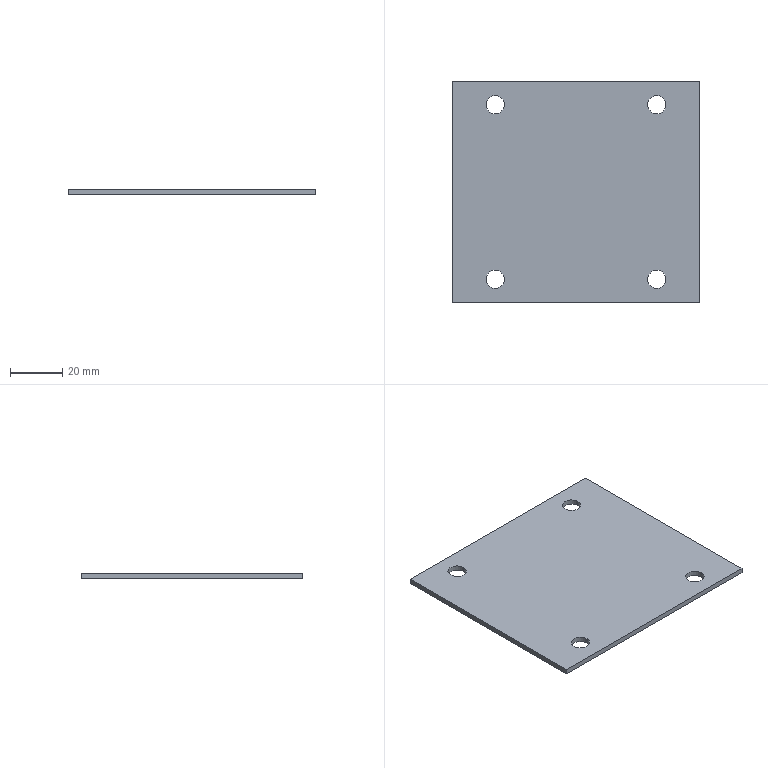Part | STEP file | GLSJ-10-47 | 1 solid | 14 faces | box 95 x 85 x 2 mm | volume 15842 mm3 | cylinder 8 | plane 6 | commonest cylinder face diameters 7 x8
STEP:
#1=CARTESIAN_POINT('',(0.,0.,0.));
#2=DIRECTION('',(0.,0.,1.));
#3=DIRECTION('',(1.,0.,0.));
#4=AXIS2_PLACEMENT_3D('',#1,#2,#3);
#5=CARTESIAN_POINT('',(-27.5,-33.5,0.));
#6=VERTEX_POINT('',#5);
#7=CARTESIAN_POINT('',(-27.5,-33.5,2.));
#8=VERTEX_POINT('',#7);
#9=CARTESIAN_POINT('',(-27.5,-33.5,0.));
#10=DIRECTION('',(0.,0.,1.));
#11=VECTOR('',#10,1.);
#12=LINE('',#9,#11);
#13=CARTESIAN_POINT('',(-31.,-33.5,0.));
#14=DIRECTION('',(0.,0.,1.));
#15=DIRECTION('',(1.,0.,0.));
#16=AXIS2_PLACEMENT_3D('',#13,#14,#15);
#17=CYLINDRICAL_SURFACE('',#16,3.5);
#18=CARTESIAN_POINT('',(6.283,0.));
#19=DIRECTION('',(0.,1.));
#20=VECTOR('',#19,1.);
#21=LINE('',#18,#20);
#22=(GEOMETRIC_REPRESENTATION_CONTEXT(2)PARAMETRIC_REPRESENTATION_CONTEXT()REPRESENTATION_CONTEXT('',''));
#23=DEFINITIONAL_REPRESENTATION('',(#21),#22);
#24=PCURVE('',#17,#23);
#25=CARTESIAN_POINT('',(-31.,-33.5,0.));
#26=DIRECTION('',(0.,0.,1.));
#27=DIRECTION('',(1.,0.,0.));
#28=AXIS2_PLACEMENT_3D('',#25,#26,#27);
#29=CYLINDRICAL_SURFACE('',#28,3.5);
#30=CARTESIAN_POINT('',(0.,0.));
#31=DIRECTION('',(0.,1.));
#32=VECTOR('',#31,1.);
#33=LINE('',#30,#32);
#34=(GEOMETRIC_REPRESENTATION_CONTEXT(2)PARAMETRIC_REPRESENTATION_CONTEXT()REPRESENTATION_CONTEXT('',''));
#35=DEFINITIONAL_REPRESENTATION('',(#33),#34);
#36=PCURVE('',#29,#35);
#37=SURFACE_CURVE('',#12,(#24,#36),.PCURVE_S1.);
#38=EDGE_CURVE('',#6,#8,#37,.T.);
#39=ORIENTED_EDGE('',*,*,#38,.T.);
#40=CARTESIAN_POINT('',(-34.5,-33.5,2.));
#41=VERTEX_POINT('',#40);
#42=CARTESIAN_POINT('',(-31.,-33.5,2.));
#43=DIRECTION('',(0.,0.,1.));
#44=DIRECTION('',(-1.,0.,0.));
#45=AXIS2_PLACEMENT_3D('',#42,#43,#44);
#46=CIRCLE('',#45,3.5);
#47=CARTESIAN_POINT('',(3.142,2.));
#48=DIRECTION('',(1.,0.));
#49=VECTOR('',#48,1.);
#50=LINE('',#47,#49);
#51=(GEOMETRIC_REPRESENTATION_CONTEXT(2)PARAMETRIC_REPRESENTATION_CONTEXT()REPRESENTATION_CONTEXT('',''));
#52=DEFINITIONAL_REPRESENTATION('',(#50),#51);
#53=PCURVE('',#17,#52);
#54=CARTESIAN_POINT('',(0.,0.,2.));
#55=DIRECTION('',(0.,0.,-1.));
#56=DIRECTION('',(-1.,0.,0.));
#57=AXIS2_PLACEMENT_3D('',#54,#55,#56);
#58=PLANE('',#57);
#59=CARTESIAN_POINT('',(34.5,-33.5));
#60=CARTESIAN_POINT('',(34.5,-39.562));
#61=CARTESIAN_POINT('',(29.25,-36.531));
#62=CARTESIAN_POINT('',(24.,-33.5));
#63=CARTESIAN_POINT('',(29.25,-30.469));
#64=CARTESIAN_POINT('',(34.5,-27.438));
#65=CARTESIAN_POINT('',(34.5,-33.5));
#66=(BOUNDED_CURVE()B_SPLINE_CURVE(2,(#59,#60,#61,#62,#63,#64,#65),.UNSPECIFIED.,.T.,.F.)B_SPLINE_CURVE_WITH_KNOTS((1,2,2,2,2,1),(-2.094,0.,2.094,4.189,6.283,8.378),.UNSPECIFIED.)CURVE()GEOMETRIC_REPRESENTATION_ITEM()RATIONAL_B_SPLINE_CURVE((1.,0.5,1.,0.5,1.,0.5,1.))REPRESENTATION_ITEM(''));
#67=(GEOMETRIC_REPRESENTATION_CONTEXT(2)PARAMETRIC_REPRESENTATION_CONTEXT()REPRESENTATION_CONTEXT('',''));
#68=DEFINITIONAL_REPRESENTATION('',(#66),#67);
#69=PCURVE('',#58,#68);
#70=SURFACE_CURVE('',#46,(#53,#69),.PCURVE_S1.);
#71=EDGE_CURVE('',#41,#8,#70,.T.);
#72=ORIENTED_EDGE('',*,*,#71,.F.);
#73=CARTESIAN_POINT('',(-34.5,-33.5,0.));
#74=VERTEX_POINT('',#73);
#75=CARTESIAN_POINT('',(-34.5,-33.5,0.));
#76=DIRECTION('',(0.,0.,1.));
#77=VECTOR('',#76,1.);
#78=LINE('',#75,#77);
#79=CARTESIAN_POINT('',(3.142,0.));
#80=DIRECTION('',(0.,1.));
#81=VECTOR('',#80,1.);
#82=LINE('',#79,#81);
#83=(GEOMETRIC_REPRESENTATION_CONTEXT(2)PARAMETRIC_REPRESENTATION_CONTEXT()REPRESENTATION_CONTEXT('',''));
#84=DEFINITIONAL_REPRESENTATION('',(#82),#83);
#85=PCURVE('',#17,#84);
#86=CARTESIAN_POINT('',(3.142,0.));
#87=DIRECTION('',(0.,1.));
#88=VECTOR('',#87,1.);
#89=LINE('',#86,#88);
#90=(GEOMETRIC_REPRESENTATION_CONTEXT(2)PARAMETRIC_REPRESENTATION_CONTEXT()REPRESENTATION_CONTEXT('',''));
#91=DEFINITIONAL_REPRESENTATION('',(#89),#90);
#92=PCURVE('',#29,#91);
#93=SURFACE_CURVE('',#78,(#85,#92),.PCURVE_S1.);
#94=EDGE_CURVE('',#74,#41,#93,.T.);
#95=ORIENTED_EDGE('',*,*,#94,.F.);
#96=CARTESIAN_POINT('',(-31.,-33.5,0.));
#97=DIRECTION('',(0.,0.,1.));
#98=DIRECTION('',(-1.,0.,0.));
#99=AXIS2_PLACEMENT_3D('',#96,#97,#98);
#100=CIRCLE('',#99,3.5);
#101=CARTESIAN_POINT('',(3.142,0.));
#102=DIRECTION('',(1.,0.));
#103=VECTOR('',#102,1.);
#104=LINE('',#101,#103);
#105=(GEOMETRIC_REPRESENTATION_CONTEXT(2)PARAMETRIC_REPRESENTATION_CONTEXT()REPRESENTATION_CONTEXT('',''));
#106=DEFINITIONAL_REPRESENTATION('',(#104),#105);
#107=PCURVE('',#17,#106);
#108=CARTESIAN_POINT('',(0.,0.,0.));
#109=DIRECTION('',(0.,0.,-1.));
#110=DIRECTION('',(-1.,0.,0.));
#111=AXIS2_PLACEMENT_3D('',#108,#109,#110);
#112=PLANE('',#111);
#113=CARTESIAN_POINT('',(34.5,-33.5));
#114=CARTESIAN_POINT('',(34.5,-39.562));
#115=CARTESIAN_POINT('',(29.25,-36.531));
#116=CARTESIAN_POINT('',(24.,-33.5));
#117=CARTESIAN_POINT('',(29.25,-30.469));
#118=CARTESIAN_POINT('',(34.5,-27.438));
#119=CARTESIAN_POINT('',(34.5,-33.5));
#120=(BOUNDED_CURVE()B_SPLINE_CURVE(2,(#113,#114,#115,#116,#117,#118,#119),.UNSPECIFIED.,.T.,.F.)B_SPLINE_CURVE_WITH_KNOTS((1,2,2,2,2,1),(-2.094,0.,2.094,4.189,6.283,8.378),.UNSPECIFIED.)CURVE()GEOMETRIC_REPRESENTATION_ITEM()RATIONAL_B_SPLINE_CURVE((1.,0.5,1.,0.5,1.,0.5,1.))REPRESENTATION_ITEM(''));
#121=(GEOMETRIC_REPRESENTATION_CONTEXT(2)PARAMETRIC_REPRESENTATION_CONTEXT()REPRESENTATION_CONTEXT('',''));
#122=DEFINITIONAL_REPRESENTATION('',(#120),#121);
#123=PCURVE('',#112,#122);
#124=SURFACE_CURVE('',#100,(#107,#123),.PCURVE_S1.);
#125=EDGE_CURVE('',#74,#6,#124,.T.);
#126=ORIENTED_EDGE('',*,*,#125,.T.);
#127=EDGE_LOOP('',(#39,#72,#95,#126));
#128=FACE_BOUND('',#127,.F.);
#129=ADVANCED_FACE('',(#128),#17,.F.);
#130=CARTESIAN_POINT('',(34.5,-33.5,0.));
#131=VERTEX_POINT('',#130);
#132=CARTESIAN_POINT('',(34.5,-33.5,2.));
#133=VERTEX_POINT('',#132);
#134=CARTESIAN_POINT('',(34.5,-33.5,0.));
#135=DIRECTION('',(0.,0.,1.));
#136=VECTOR('',#135,1.);
#137=LINE('',#134,#136);
#138=CARTESIAN_POINT('',(31.,-33.5,0.));
#139=DIRECTION('',(0.,0.,1.));
#140=DIRECTION('',(1.,0.,0.));
#141=AXIS2_PLACEMENT_3D('',#138,#139,#140);
#142=CYLINDRICAL_SURFACE('',#141,3.5);
#143=CARTESIAN_POINT('',(6.283,0.));
#144=DIRECTION('',(0.,1.));
#145=VECTOR('',#144,1.);
#146=LINE('',#143,#145);
#147=(GEOMETRIC_REPRESENTATION_CONTEXT(2)PARAMETRIC_REPRESENTATION_CONTEXT()REPRESENTATION_CONTEXT('',''));
#148=DEFINITIONAL_REPRESENTATION('',(#146),#147);
#149=PCURVE('',#142,#148);
#150=CARTESIAN_POINT('',(31.,-33.5,0.));
#151=DIRECTION('',(0.,0.,1.));
#152=DIRECTION('',(1.,0.,0.));
#153=AXIS2_PLACEMENT_3D('',#150,#151,#152);
#154=CYLINDRICAL_SURFACE('',#153,3.5);
#155=CARTESIAN_POINT('',(0.,0.));
#156=DIRECTION('',(0.,1.));
#157=VECTOR('',#156,1.);
#158=LINE('',#155,#157);
#159=(GEOMETRIC_REPRESENTATION_CONTEXT(2)PARAMETRIC_REPRESENTATION_CONTEXT()REPRESENTATION_CONTEXT('',''));
#160=DEFINITIONAL_REPRESENTATION('',(#158),#159);
#161=PCURVE('',#154,#160);
#162=SURFACE_CURVE('',#137,(#149,#161),.PCURVE_S1.);
#163=EDGE_CURVE('',#131,#133,#162,.T.);
#164=ORIENTED_EDGE('',*,*,#163,.T.);
#165=CARTESIAN_POINT('',(27.5,-33.5,2.));
#166=VERTEX_POINT('',#165);
#167=CARTESIAN_POINT('',(31.,-33.5,2.));
#168=DIRECTION('',(0.,0.,1.));
#169=DIRECTION('',(1.,0.,0.));
#170=AXIS2_PLACEMENT_3D('',#167,#168,#169);
#171=CIRCLE('',#170,3.5);
#172=CARTESIAN_POINT('',(0.,2.));
#173=DIRECTION('',(1.,0.));
#174=VECTOR('',#173,1.);
#175=LINE('',#172,#174);
#176=(GEOMETRIC_REPRESENTATION_CONTEXT(2)PARAMETRIC_REPRESENTATION_CONTEXT()REPRESENTATION_CONTEXT('',''));
#177=DEFINITIONAL_REPRESENTATION('',(#175),#176);
#178=PCURVE('',#142,#177);
#179=CARTESIAN_POINT('',(-34.5,-33.5));
#180=CARTESIAN_POINT('',(-34.5,-27.438));
#181=CARTESIAN_POINT('',(-29.25,-30.469));
#182=CARTESIAN_POINT('',(-24.,-33.5));
#183=CARTESIAN_POINT('',(-29.25,-36.531));
#184=CARTESIAN_POINT('',(-34.5,-39.562));
#185=CARTESIAN_POINT('',(-34.5,-33.5));
#186=(BOUNDED_CURVE()B_SPLINE_CURVE(2,(#179,#180,#181,#182,#183,#184,#185),.UNSPECIFIED.,.T.,.F.)B_SPLINE_CURVE_WITH_KNOTS((1,2,2,2,2,1),(-2.094,0.,2.094,4.189,6.283,8.378),.UNSPECIFIED.)CURVE()GEOMETRIC_REPRESENTATION_ITEM()RATIONAL_B_SPLINE_CURVE((1.,0.5,1.,0.5,1.,0.5,1.))REPRESENTATION_ITEM(''));
#187=(GEOMETRIC_REPRESENTATION_CONTEXT(2)PARAMETRIC_REPRESENTATION_CONTEXT()REPRESENTATION_CONTEXT('',''));
#188=DEFINITIONAL_REPRESENTATION('',(#186),#187);
#189=PCURVE('',#58,#188);
#190=SURFACE_CURVE('',#171,(#178,#189),.PCURVE_S1.);
#191=EDGE_CURVE('',#166,#133,#190,.T.);
#192=ORIENTED_EDGE('',*,*,#191,.F.);
#193=CARTESIAN_POINT('',(27.5,-33.5,0.));
#194=VERTEX_POINT('',#193);
#195=CARTESIAN_POINT('',(27.5,-33.5,0.));
#196=DIRECTION('',(0.,0.,1.));
#197=VECTOR('',#196,1.);
#198=LINE('',#195,#197);
#199=CARTESIAN_POINT('',(3.142,0.));
#200=DIRECTION('',(0.,1.));
#201=VECTOR('',#200,1.);
#202=LINE('',#199,#201);
#203=(GEOMETRIC_REPRESENTATION_CONTEXT(2)PARAMETRIC_REPRESENTATION_CONTEXT()REPRESENTATION_CONTEXT('',''));
#204=DEFINITIONAL_REPRESENTATION('',(#202),#203);
#205=PCURVE('',#142,#204);
#206=CARTESIAN_POINT('',(3.142,0.));
#207=DIRECTION('',(0.,1.));
#208=VECTOR('',#207,1.);
#209=LINE('',#206,#208);
#210=(GEOMETRIC_REPRESENTATION_CONTEXT(2)PARAMETRIC_REPRESENTATION_CONTEXT()REPRESENTATION_CONTEXT('',''));
#211=DEFINITIONAL_REPRESENTATION('',(#209),#210);
#212=PCURVE('',#154,#211);
#213=SURFACE_CURVE('',#198,(#205,#212),.PCURVE_S1.);
#214=EDGE_CURVE('',#194,#166,#213,.T.);
#215=ORIENTED_EDGE('',*,*,#214,.F.);
#216=CARTESIAN_POINT('',(31.,-33.5,0.));
#217=DIRECTION('',(0.,0.,1.));
#218=DIRECTION('',(1.,0.,0.));
#219=AXIS2_PLACEMENT_3D('',#216,#217,#218);
#220=CIRCLE('',#219,3.5);
#221=CARTESIAN_POINT('',(0.,0.));
#222=DIRECTION('',(1.,0.));
#223=VECTOR('',#222,1.);
#224=LINE('',#221,#223);
#225=(GEOMETRIC_REPRESENTATION_CONTEXT(2)PARAMETRIC_REPRESENTATION_CONTEXT()REPRESENTATION_CONTEXT('',''));
#226=DEFINITIONAL_REPRESENTATION('',(#224),#225);
#227=PCURVE('',#142,#226);
#228=CARTESIAN_POINT('',(-34.5,-33.5));
#229=CARTESIAN_POINT('',(-34.5,-27.438));
#230=CARTESIAN_POINT('',(-29.25,-30.469));
#231=CARTESIAN_POINT('',(-24.,-33.5));
#232=CARTESIAN_POINT('',(-29.25,-36.531));
#233=CARTESIAN_POINT('',(-34.5,-39.562));
#234=CARTESIAN_POINT('',(-34.5,-33.5));
#235=(BOUNDED_CURVE()B_SPLINE_CURVE(2,(#228,#229,#230,#231,#232,#233,#234),.UNSPECIFIED.,.T.,.F.)B_SPLINE_CURVE_WITH_KNOTS((1,2,2,2,2,1),(-2.094,0.,2.094,4.189,6.283,8.378),.UNSPECIFIED.)CURVE()GEOMETRIC_REPRESENTATION_ITEM()RATIONAL_B_SPLINE_CURVE((1.,0.5,1.,0.5,1.,0.5,1.))REPRESENTATION_ITEM(''));
#236=(GEOMETRIC_REPRESENTATION_CONTEXT(2)PARAMETRIC_REPRESENTATION_CONTEXT()REPRESENTATION_CONTEXT('',''));
#237=DEFINITIONAL_REPRESENTATION('',(#235),#236);
#238=PCURVE('',#112,#237);
#239=SURFACE_CURVE('',#220,(#227,#238),.PCURVE_S1.);
#240=EDGE_CURVE('',#194,#131,#239,.T.);
#241=ORIENTED_EDGE('',*,*,#240,.T.);
#242=EDGE_LOOP('',(#164,#192,#215,#241));
#243=FACE_BOUND('',#242,.F.);
#244=ADVANCED_FACE('',(#243),#142,.F.);
#245=CARTESIAN_POINT('',(34.5,33.5,0.));
#246=VERTEX_POINT('',#245);
#247=CARTESIAN_POINT('',(34.5,33.5,2.));
#248=VERTEX_POINT('',#247);
#249=CARTESIAN_POINT('',(34.5,33.5,0.));
#250=DIRECTION('',(0.,0.,1.));
#251=VECTOR('',#250,1.);
#252=LINE('',#249,#251);
#253=CARTESIAN_POINT('',(31.,33.5,0.));
#254=DIRECTION('',(0.,0.,1.));
#255=DIRECTION('',(1.,0.,0.));
#256=AXIS2_PLACEMENT_3D('',#253,#254,#255);
#257=CYLINDRICAL_SURFACE('',#256,3.5);
#258=CARTESIAN_POINT('',(6.283,0.));
#259=DIRECTION('',(0.,1.));
#260=VECTOR('',#259,1.);
#261=LINE('',#258,#260);
#262=(GEOMETRIC_REPRESENTATION_CONTEXT(2)PARAMETRIC_REPRESENTATION_CONTEXT()REPRESENTATION_CONTEXT('',''));
#263=DEFINITIONAL_REPRESENTATION('',(#261),#262);
#264=PCURVE('',#257,#263);
#265=CARTESIAN_POINT('',(31.,33.5,0.));
#266=DIRECTION('',(0.,0.,1.));
#267=DIRECTION('',(1.,0.,0.));
#268=AXIS2_PLACEMENT_3D('',#265,#266,#267);
#269=CYLINDRICAL_SURFACE('',#268,3.5);
#270=CARTESIAN_POINT('',(0.,0.));
#271=DIRECTION('',(0.,1.));
#272=VECTOR('',#271,1.);
#273=LINE('',#270,#272);
#274=(GEOMETRIC_REPRESENTATION_CONTEXT(2)PARAMETRIC_REPRESENTATION_CONTEXT()REPRESENTATION_CONTEXT('',''));
#275=DEFINITIONAL_REPRESENTATION('',(#273),#274);
#276=PCURVE('',#269,#275);
#277=SURFACE_CURVE('',#252,(#264,#276),.PCURVE_S1.);
#278=EDGE_CURVE('',#246,#248,#277,.T.);
#279=ORIENTED_EDGE('',*,*,#278,.T.);
#280=CARTESIAN_POINT('',(27.5,33.5,2.));
#281=VERTEX_POINT('',#280);
#282=CARTESIAN_POINT('',(31.,33.5,2.));
#283=DIRECTION('',(0.,0.,1.));
#284=DIRECTION('',(-1.,0.,0.));
#285=AXIS2_PLACEMENT_3D('',#282,#283,#284);
#286=CIRCLE('',#285,3.5);
#287=CARTESIAN_POINT('',(3.142,2.));
#288=DIRECTION('',(1.,0.));
#289=VECTOR('',#288,1.);
#290=LINE('',#287,#289);
#291=(GEOMETRIC_REPRESENTATION_CONTEXT(2)PARAMETRIC_REPRESENTATION_CONTEXT()REPRESENTATION_CONTEXT('',''));
#292=DEFINITIONAL_REPRESENTATION('',(#290),#291);
#293=PCURVE('',#257,#292);
#294=CARTESIAN_POINT('',(-27.5,33.5));
#295=CARTESIAN_POINT('',(-27.5,27.438));
#296=CARTESIAN_POINT('',(-32.75,30.469));
#297=CARTESIAN_POINT('',(-38.,33.5));
#298=CARTESIAN_POINT('',(-32.75,36.531));
#299=CARTESIAN_POINT('',(-27.5,39.562));
#300=CARTESIAN_POINT('',(-27.5,33.5));
#301=(BOUNDED_CURVE()B_SPLINE_CURVE(2,(#294,#295,#296,#297,#298,#299,#300),.UNSPECIFIED.,.T.,.F.)B_SPLINE_CURVE_WITH_KNOTS((1,2,2,2,2,1),(-2.094,0.,2.094,4.189,6.283,8.378),.UNSPECIFIED.)CURVE()GEOMETRIC_REPRESENTATION_ITEM()RATIONAL_B_SPLINE_CURVE((1.,0.5,1.,0.5,1.,0.5,1.))REPRESENTATION_ITEM(''));
#302=(GEOMETRIC_REPRESENTATION_CONTEXT(2)PARAMETRIC_REPRESENTATION_CONTEXT()REPRESENTATION_CONTEXT('',''));
#303=DEFINITIONAL_REPRESENTATION('',(#301),#302);
#304=PCURVE('',#58,#303);
#305=SURFACE_CURVE('',#286,(#293,#304),.PCURVE_S1.);
#306=EDGE_CURVE('',#281,#248,#305,.T.);
#307=ORIENTED_EDGE('',*,*,#306,.F.);
#308=CARTESIAN_POINT('',(27.5,33.5,0.));
#309=VERTEX_POINT('',#308);
#310=CARTESIAN_POINT('',(27.5,33.5,0.));
#311=DIRECTION('',(0.,0.,1.));
#312=VECTOR('',#311,1.);
#313=LINE('',#310,#312);
#314=CARTESIAN_POINT('',(3.142,0.));
#315=DIRECTION('',(0.,1.));
#316=VECTOR('',#315,1.);
#317=LINE('',#314,#316);
#318=(GEOMETRIC_REPRESENTATION_CONTEXT(2)PARAMETRIC_REPRESENTATION_CONTEXT()REPRESENTATION_CONTEXT('',''));
#319=DEFINITIONAL_REPRESENTATION('',(#317),#318);
#320=PCURVE('',#257,#319);
#321=CARTESIAN_POINT('',(3.142,0.));
#322=DIRECTION('',(0.,1.));
#323=VECTOR('',#322,1.);
#324=LINE('',#321,#323);
#325=(GEOMETRIC_REPRESENTATION_CONTEXT(2)PARAMETRIC_REPRESENTATION_CONTEXT()REPRESENTATION_CONTEXT('',''));
#326=DEFINITIONAL_REPRESENTATION('',(#324),#325);
#327=PCURVE('',#269,#326);
#328=SURFACE_CURVE('',#313,(#320,#327),.PCURVE_S1.);
#329=EDGE_CURVE('',#309,#281,#328,.T.);
#330=ORIENTED_EDGE('',*,*,#329,.F.);
#331=CARTESIAN_POINT('',(31.,33.5,0.));
#332=DIRECTION('',(0.,0.,1.));
#333=DIRECTION('',(-1.,0.,0.));
#334=AXIS2_PLACEMENT_3D('',#331,#332,#333);
#335=CIRCLE('',#334,3.5);
#336=CARTESIAN_POINT('',(3.142,0.));
#337=DIRECTION('',(1.,0.));
#338=VECTOR('',#337,1.);
#339=LINE('',#336,#338);
#340=(GEOMETRIC_REPRESENTATION_CONTEXT(2)PARAMETRIC_REPRESENTATION_CONTEXT()REPRESENTATION_CONTEXT('',''));
#341=DEFINITIONAL_REPRESENTATION('',(#339),#340);
#342=PCURVE('',#257,#341);
#343=CARTESIAN_POINT('',(-27.5,33.5));
#344=CARTESIAN_POINT('',(-27.5,27.438));
#345=CARTESIAN_POINT('',(-32.75,30.469));
#346=CARTESIAN_POINT('',(-38.,33.5));
#347=CARTESIAN_POINT('',(-32.75,36.531));
#348=CARTESIAN_POINT('',(-27.5,39.562));
#349=CARTESIAN_POINT('',(-27.5,33.5));
#350=(BOUNDED_CURVE()B_SPLINE_CURVE(2,(#343,#344,#345,#346,#347,#348,#349),.UNSPECIFIED.,.T.,.F.)B_SPLINE_CURVE_WITH_KNOTS((1,2,2,2,2,1),(-2.094,0.,2.094,4.189,6.283,8.378),.UNSPECIFIED.)CURVE()GEOMETRIC_REPRESENTATION_ITEM()RATIONAL_B_SPLINE_CURVE((1.,0.5,1.,0.5,1.,0.5,1.))REPRESENTATION_ITEM(''));
#351=(GEOMETRIC_REPRESENTATION_CONTEXT(2)PARAMETRIC_REPRESENTATION_CONTEXT()REPRESENTATION_CONTEXT('',''));
#352=DEFINITIONAL_REPRESENTATION('',(#350),#351);
#353=PCURVE('',#112,#352);
#354=SURFACE_CURVE('',#335,(#342,#353),.PCURVE_S1.);
#355=EDGE_CURVE('',#309,#246,#354,.T.);
#356=ORIENTED_EDGE('',*,*,#355,.T.);
#357=EDGE_LOOP('',(#279,#307,#330,#356));
#358=FACE_BOUND('',#357,.F.);
#359=ADVANCED_FACE('',(#358),#257,.F.);
#360=CARTESIAN_POINT('',(-27.5,33.5,0.));
#361=VERTEX_POINT('',#360);
#362=CARTESIAN_POINT('',(-27.5,33.5,2.));
#363=VERTEX_POINT('',#362);
#364=CARTESIAN_POINT('',(-27.5,33.5,0.));
#365=DIRECTION('',(0.,0.,1.));
#366=VECTOR('',#365,1.);
#367=LINE('',#364,#366);
#368=CARTESIAN_POINT('',(-31.,33.5,0.));
#369=DIRECTION('',(0.,0.,1.));
#370=DIRECTION('',(1.,0.,0.));
#371=AXIS2_PLACEMENT_3D('',#368,#369,#370);
#372=CYLINDRICAL_SURFACE('',#371,3.5);
#373=CARTESIAN_POINT('',(6.283,0.));
#374=DIRECTION('',(0.,1.));
#375=VECTOR('',#374,1.);
#376=LINE('',#373,#375);
#377=(GEOMETRIC_REPRESENTATION_CONTEXT(2)PARAMETRIC_REPRESENTATION_CONTEXT()REPRESENTATION_CONTEXT('',''));
#378=DEFINITIONAL_REPRESENTATION('',(#376),#377);
#379=PCURVE('',#372,#378);
#380=CARTESIAN_POINT('',(-31.,33.5,0.));
#381=DIRECTION('',(0.,0.,1.));
#382=DIRECTION('',(1.,0.,0.));
#383=AXIS2_PLACEMENT_3D('',#380,#381,#382);
#384=CYLINDRICAL_SURFACE('',#383,3.5);
#385=CARTESIAN_POINT('',(0.,0.));
#386=DIRECTION('',(0.,1.));
#387=VECTOR('',#386,1.);
#388=LINE('',#385,#387);
#389=(GEOMETRIC_REPRESENTATION_CONTEXT(2)PARAMETRIC_REPRESENTATION_CONTEXT()REPRESENTATION_CONTEXT('',''));
#390=DEFINITIONAL_REPRESENTATION('',(#388),#389);
#391=PCURVE('',#384,#390);
#392=SURFACE_CURVE('',#367,(#379,#391),.PCURVE_S1.);
#393=EDGE_CURVE('',#361,#363,#392,.T.);
#394=ORIENTED_EDGE('',*,*,#393,.T.);
#395=CARTESIAN_POINT('',(-34.5,33.5,2.));
#396=VERTEX_POINT('',#395);
#397=CARTESIAN_POINT('',(-31.,33.5,2.));
#398=DIRECTION('',(0.,0.,1.));
#399=DIRECTION('',(1.,0.,0.));
#400=AXIS2_PLACEMENT_3D('',#397,#398,#399);
#401=CIRCLE('',#400,3.5);
#402=CARTESIAN_POINT('',(0.,2.));
#403=DIRECTION('',(1.,0.));
#404=VECTOR('',#403,1.);
#405=LINE('',#402,#404);
#406=(GEOMETRIC_REPRESENTATION_CONTEXT(2)PARAMETRIC_REPRESENTATION_CONTEXT()REPRESENTATION_CONTEXT('',''));
#407=DEFINITIONAL_REPRESENTATION('',(#405),#406);
#408=PCURVE('',#372,#407);
#409=CARTESIAN_POINT('',(27.5,33.5));
#410=CARTESIAN_POINT('',(27.5,39.562));
#411=CARTESIAN_POINT('',(32.75,36.531));
#412=CARTESIAN_POINT('',(38.,33.5));
#413=CARTESIAN_POINT('',(32.75,30.469));
#414=CARTESIAN_POINT('',(27.5,27.438));
#415=CARTESIAN_POINT('',(27.5,33.5));
#416=(BOUNDED_CURVE()B_SPLINE_CURVE(2,(#409,#410,#411,#412,#413,#414,#415),.UNSPECIFIED.,.T.,.F.)B_SPLINE_CURVE_WITH_KNOTS((1,2,2,2,2,1),(-2.094,0.,2.094,4.189,6.283,8.378),.UNSPECIFIED.)CURVE()GEOMETRIC_REPRESENTATION_ITEM()RATIONAL_B_SPLINE_CURVE((1.,0.5,1.,0.5,1.,0.5,1.))REPRESENTATION_ITEM(''));
#417=(GEOMETRIC_REPRESENTATION_CONTEXT(2)PARAMETRIC_REPRESENTATION_CONTEXT()REPRESENTATION_CONTEXT('',''));
#418=DEFINITIONAL_REPRESENTATION('',(#416),#417);
#419=PCURVE('',#58,#418);
#420=SURFACE_CURVE('',#401,(#408,#419),.PCURVE_S1.);
#421=EDGE_CURVE('',#396,#363,#420,.T.);
#422=ORIENTED_EDGE('',*,*,#421,.F.);
#423=CARTESIAN_POINT('',(-34.5,33.5,0.));
#424=VERTEX_POINT('',#423);
#425=CARTESIAN_POINT('',(-34.5,33.5,0.));
#426=DIRECTION('',(0.,0.,1.));
#427=VECTOR('',#426,1.);
#428=LINE('',#425,#427);
#429=CARTESIAN_POINT('',(3.142,0.));
#430=DIRECTION('',(0.,1.));
#431=VECTOR('',#430,1.);
#432=LINE('',#429,#431);
#433=(GEOMETRIC_REPRESENTATION_CONTEXT(2)PARAMETRIC_REPRESENTATION_CONTEXT()REPRESENTATION_CONTEXT('',''));
#434=DEFINITIONAL_REPRESENTATION('',(#432),#433);
#435=PCURVE('',#372,#434);
#436=CARTESIAN_POINT('',(3.142,0.));
#437=DIRECTION('',(0.,1.));
#438=VECTOR('',#437,1.);
#439=LINE('',#436,#438);
#440=(GEOMETRIC_REPRESENTATION_CONTEXT(2)PARAMETRIC_REPRESENTATION_CONTEXT()REPRESENTATION_CONTEXT('',''));
#441=DEFINITIONAL_REPRESENTATION('',(#439),#440);
#442=PCURVE('',#384,#441);
#443=SURFACE_CURVE('',#428,(#435,#442),.PCURVE_S1.);
#444=EDGE_CURVE('',#424,#396,#443,.T.);
#445=ORIENTED_EDGE('',*,*,#444,.F.);
#446=CARTESIAN_POINT('',(-31.,33.5,0.));
#447=DIRECTION('',(0.,0.,1.));
#448=DIRECTION('',(1.,0.,0.));
#449=AXIS2_PLACEMENT_3D('',#446,#447,#448);
#450=CIRCLE('',#449,3.5);
#451=CARTESIAN_POINT('',(0.,0.));
#452=DIRECTION('',(1.,0.));
#453=VECTOR('',#452,1.);
#454=LINE('',#451,#453);
#455=(GEOMETRIC_REPRESENTATION_CONTEXT(2)PARAMETRIC_REPRESENTATION_CONTEXT()REPRESENTATION_CONTEXT('',''));
#456=DEFINITIONAL_REPRESENTATION('',(#454),#455);
#457=PCURVE('',#372,#456);
#458=CARTESIAN_POINT('',(27.5,33.5));
#459=CARTESIAN_POINT('',(27.5,39.562));
#460=CARTESIAN_POINT('',(32.75,36.531));
#461=CARTESIAN_POINT('',(38.,33.5));
#462=CARTESIAN_POINT('',(32.75,30.469));
#463=CARTESIAN_POINT('',(27.5,27.438));
#464=CARTESIAN_POINT('',(27.5,33.5));
#465=(BOUNDED_CURVE()B_SPLINE_CURVE(2,(#458,#459,#460,#461,#462,#463,#464),.UNSPECIFIED.,.T.,.F.)B_SPLINE_CURVE_WITH_KNOTS((1,2,2,2,2,1),(-2.094,0.,2.094,4.189,6.283,8.378),.UNSPECIFIED.)CURVE()GEOMETRIC_REPRESENTATION_ITEM()RATIONAL_B_SPLINE_CURVE((1.,0.5,1.,0.5,1.,0.5,1.))REPRESENTATION_ITEM(''));
#466=(GEOMETRIC_REPRESENTATION_CONTEXT(2)PARAMETRIC_REPRESENTATION_CONTEXT()REPRESENTATION_CONTEXT('',''));
#467=DEFINITIONAL_REPRESENTATION('',(#465),#466);
#468=PCURVE('',#112,#467);
#469=SURFACE_CURVE('',#450,(#457,#468),.PCURVE_S1.);
#470=EDGE_CURVE('',#424,#361,#469,.T.);
#471=ORIENTED_EDGE('',*,*,#470,.T.);
#472=EDGE_LOOP('',(#394,#422,#445,#471));
#473=FACE_BOUND('',#472,.F.);
#474=ADVANCED_FACE('',(#473),#372,.F.);
#475=CARTESIAN_POINT('',(-47.5,42.5,0.));
#476=VERTEX_POINT('',#475);
#477=CARTESIAN_POINT('',(-47.5,-42.5,0.));
#478=VERTEX_POINT('',#477);
#479=CARTESIAN_POINT('',(-47.5,42.5,0.));
#480=DIRECTION('',(0.,-1.,0.));
#481=VECTOR('',#480,1.);
#482=LINE('',#479,#481);
#483=CARTESIAN_POINT('',(-47.5,42.5,2.));
#484=DIRECTION('',(1.,0.,0.));
#485=DIRECTION('',(0.,1.,0.));
#486=AXIS2_PLACEMENT_3D('',#483,#484,#485);
#487=PLANE('',#486);
#488=CARTESIAN_POINT('',(0.,-2.));
#489=DIRECTION('',(-1.,0.));
#490=VECTOR('',#489,1.);
#491=LINE('',#488,#490);
#492=(GEOMETRIC_REPRESENTATION_CONTEXT(2)PARAMETRIC_REPRESENTATION_CONTEXT()REPRESENTATION_CONTEXT('',''));
#493=DEFINITIONAL_REPRESENTATION('',(#491),#492);
#494=PCURVE('',#487,#493);
#495=CARTESIAN_POINT('',(47.5,42.5));
#496=DIRECTION('',(0.,-1.));
#497=VECTOR('',#496,1.);
#498=LINE('',#495,#497);
#499=(GEOMETRIC_REPRESENTATION_CONTEXT(2)PARAMETRIC_REPRESENTATION_CONTEXT()REPRESENTATION_CONTEXT('',''));
#500=DEFINITIONAL_REPRESENTATION('',(#498),#499);
#501=PCURVE('',#112,#500);
#502=SURFACE_CURVE('',#482,(#494,#501),.PCURVE_S1.);
#503=EDGE_CURVE('',#476,#478,#502,.T.);
#504=ORIENTED_EDGE('',*,*,#503,.T.);
#505=CARTESIAN_POINT('',(-47.5,-42.5,2.));
#506=VERTEX_POINT('',#505);
#507=CARTESIAN_POINT('',(-47.5,-42.5,2.));
#508=DIRECTION('',(0.,0.,-1.));
#509=VECTOR('',#508,1.);
#510=LINE('',#507,#509);
#511=CARTESIAN_POINT('',(-85.,0.));
#512=DIRECTION('',(0.,-1.));
#513=VECTOR('',#512,1.);
#514=LINE('',#511,#513);
#515=(GEOMETRIC_REPRESENTATION_CONTEXT(2)PARAMETRIC_REPRESENTATION_CONTEXT()REPRESENTATION_CONTEXT('',''));
#516=DEFINITIONAL_REPRESENTATION('',(#514),#515);
#517=PCURVE('',#487,#516);
#518=CARTESIAN_POINT('',(47.5,-42.5,2.));
#519=DIRECTION('',(0.,1.,0.));
#520=DIRECTION('',(-1.,0.,0.));
#521=AXIS2_PLACEMENT_3D('',#518,#519,#520);
#522=PLANE('',#521);
#523=CARTESIAN_POINT('',(95.,0.));
#524=DIRECTION('',(0.,-1.));
#525=VECTOR('',#524,1.);
#526=LINE('',#523,#525);
#527=(GEOMETRIC_REPRESENTATION_CONTEXT(2)PARAMETRIC_REPRESENTATION_CONTEXT()REPRESENTATION_CONTEXT('',''));
#528=DEFINITIONAL_REPRESENTATION('',(#526),#527);
#529=PCURVE('',#522,#528);
#530=SURFACE_CURVE('',#510,(#517,#529),.PCURVE_S1.);
#531=EDGE_CURVE('',#506,#478,#530,.T.);
#532=ORIENTED_EDGE('',*,*,#531,.F.);
#533=CARTESIAN_POINT('',(-47.5,42.5,2.));
#534=VERTEX_POINT('',#533);
#535=CARTESIAN_POINT('',(-47.5,42.5,2.));
#536=DIRECTION('',(0.,-1.,0.));
#537=VECTOR('',#536,1.);
#538=LINE('',#535,#537);
#539=CARTESIAN_POINT('',(0.,0.));
#540=DIRECTION('',(-1.,0.));
#541=VECTOR('',#540,1.);
#542=LINE('',#539,#541);
#543=(GEOMETRIC_REPRESENTATION_CONTEXT(2)PARAMETRIC_REPRESENTATION_CONTEXT()REPRESENTATION_CONTEXT('',''));
#544=DEFINITIONAL_REPRESENTATION('',(#542),#543);
#545=PCURVE('',#487,#544);
#546=CARTESIAN_POINT('',(47.5,42.5));
#547=DIRECTION('',(0.,-1.));
#548=VECTOR('',#547,1.);
#549=LINE('',#546,#548);
#550=(GEOMETRIC_REPRESENTATION_CONTEXT(2)PARAMETRIC_REPRESENTATION_CONTEXT()REPRESENTATION_CONTEXT('',''));
#551=DEFINITIONAL_REPRESENTATION('',(#549),#550);
#552=PCURVE('',#58,#551);
#553=SURFACE_CURVE('',#538,(#545,#552),.PCURVE_S1.);
#554=EDGE_CURVE('',#534,#506,#553,.T.);
#555=ORIENTED_EDGE('',*,*,#554,.F.);
#556=CARTESIAN_POINT('',(-47.5,42.5,2.));
#557=DIRECTION('',(0.,0.,-1.));
#558=VECTOR('',#557,1.);
#559=LINE('',#556,#558);
#560=CARTESIAN_POINT('',(0.,0.));
#561=DIRECTION('',(0.,-1.));
#562=VECTOR('',#561,1.);
#563=LINE('',#560,#562);
#564=(GEOMETRIC_REPRESENTATION_CONTEXT(2)PARAMETRIC_REPRESENTATION_CONTEXT()REPRESENTATION_CONTEXT('',''));
#565=DEFINITIONAL_REPRESENTATION('',(#563),#564);
#566=PCURVE('',#487,#565);
#567=CARTESIAN_POINT('',(47.5,42.5,2.));
#568=DIRECTION('',(0.,-1.,0.));
#569=DIRECTION('',(1.,0.,0.));
#570=AXIS2_PLACEMENT_3D('',#567,#568,#569);
#571=PLANE('',#570);
#572=CARTESIAN_POINT('',(-95.,0.));
#573=DIRECTION('',(0.,-1.));
#574=VECTOR('',#573,1.);
#575=LINE('',#572,#574);
#576=(GEOMETRIC_REPRESENTATION_CONTEXT(2)PARAMETRIC_REPRESENTATION_CONTEXT()REPRESENTATION_CONTEXT('',''));
#577=DEFINITIONAL_REPRESENTATION('',(#575),#576);
#578=PCURVE('',#571,#577);
#579=SURFACE_CURVE('',#559,(#566,#578),.PCURVE_S1.);
#580=EDGE_CURVE('',#534,#476,#579,.T.);
#581=ORIENTED_EDGE('',*,*,#580,.T.);
#582=EDGE_LOOP('',(#504,#532,#555,#581));
#583=FACE_BOUND('',#582,.T.);
#584=ADVANCED_FACE('',(#583),#487,.F.);
#585=CARTESIAN_POINT('',(47.5,-42.5,0.));
#586=VERTEX_POINT('',#585);
#587=CARTESIAN_POINT('',(47.5,-42.5,0.));
#588=DIRECTION('',(1.,0.,0.));
#589=VECTOR('',#588,1.);
#590=LINE('',#587,#589);
#591=CARTESIAN_POINT('',(0.,-2.));
#592=DIRECTION('',(-1.,0.));
#593=VECTOR('',#592,1.);
#594=LINE('',#591,#593);
#595=(GEOMETRIC_REPRESENTATION_CONTEXT(2)PARAMETRIC_REPRESENTATION_CONTEXT()REPRESENTATION_CONTEXT('',''));
#596=DEFINITIONAL_REPRESENTATION('',(#594),#595);
#597=PCURVE('',#522,#596);
#598=CARTESIAN_POINT('',(-47.5,-42.5));
#599=DIRECTION('',(-1.,0.));
#600=VECTOR('',#599,1.);
#601=LINE('',#598,#600);
#602=(GEOMETRIC_REPRESENTATION_CONTEXT(2)PARAMETRIC_REPRESENTATION_CONTEXT()REPRESENTATION_CONTEXT('',''));
#603=DEFINITIONAL_REPRESENTATION('',(#601),#602);
#604=PCURVE('',#112,#603);
#605=SURFACE_CURVE('',#590,(#597,#604),.PCURVE_S1.);
#606=EDGE_CURVE('',#478,#586,#605,.T.);
#607=ORIENTED_EDGE('',*,*,#606,.T.);
#608=CARTESIAN_POINT('',(47.5,-42.5,2.));
#609=VERTEX_POINT('',#608);
#610=CARTESIAN_POINT('',(47.5,-42.5,2.));
#611=DIRECTION('',(0.,0.,-1.));
#612=VECTOR('',#611,1.);
#613=LINE('',#610,#612);
#614=CARTESIAN_POINT('',(0.,0.));
#615=DIRECTION('',(0.,-1.));
#616=VECTOR('',#615,1.);
#617=LINE('',#614,#616);
#618=(GEOMETRIC_REPRESENTATION_CONTEXT(2)PARAMETRIC_REPRESENTATION_CONTEXT()REPRESENTATION_CONTEXT('',''));
#619=DEFINITIONAL_REPRESENTATION('',(#617),#618);
#620=PCURVE('',#522,#619);
#621=CARTESIAN_POINT('',(47.5,42.5,2.));
#622=DIRECTION('',(-1.,0.,0.));
#623=DIRECTION('',(0.,-1.,0.));
#624=AXIS2_PLACEMENT_3D('',#621,#622,#623);
#625=PLANE('',#624);
#626=CARTESIAN_POINT('',(85.,0.));
#627=DIRECTION('',(0.,-1.));
#628=VECTOR('',#627,1.);
#629=LINE('',#626,#628);
#630=(GEOMETRIC_REPRESENTATION_CONTEXT(2)PARAMETRIC_REPRESENTATION_CONTEXT()REPRESENTATION_CONTEXT('',''));
#631=DEFINITIONAL_REPRESENTATION('',(#629),#630);
#632=PCURVE('',#625,#631);
#633=SURFACE_CURVE('',#613,(#620,#632),.PCURVE_S1.);
#634=EDGE_CURVE('',#609,#586,#633,.T.);
#635=ORIENTED_EDGE('',*,*,#634,.F.);
#636=CARTESIAN_POINT('',(47.5,-42.5,2.));
#637=DIRECTION('',(1.,0.,0.));
#638=VECTOR('',#637,1.);
#639=LINE('',#636,#638);
#640=CARTESIAN_POINT('',(0.,0.));
#641=DIRECTION('',(-1.,0.));
#642=VECTOR('',#641,1.);
#643=LINE('',#640,#642);
#644=(GEOMETRIC_REPRESENTATION_CONTEXT(2)PARAMETRIC_REPRESENTATION_CONTEXT()REPRESENTATION_CONTEXT('',''));
#645=DEFINITIONAL_REPRESENTATION('',(#643),#644);
#646=PCURVE('',#522,#645);
#647=CARTESIAN_POINT('',(-47.5,-42.5));
#648=DIRECTION('',(-1.,0.));
#649=VECTOR('',#648,1.);
#650=LINE('',#647,#649);
#651=(GEOMETRIC_REPRESENTATION_CONTEXT(2)PARAMETRIC_REPRESENTATION_CONTEXT()REPRESENTATION_CONTEXT('',''));
#652=DEFINITIONAL_REPRESENTATION('',(#650),#651);
#653=PCURVE('',#58,#652);
#654=SURFACE_CURVE('',#639,(#646,#653),.PCURVE_S1.);
#655=EDGE_CURVE('',#506,#609,#654,.T.);
#656=ORIENTED_EDGE('',*,*,#655,.F.);
#657=ORIENTED_EDGE('',*,*,#531,.T.);
#658=EDGE_LOOP('',(#607,#635,#656,#657));
#659=FACE_BOUND('',#658,.T.);
#660=ADVANCED_FACE('',(#659),#522,.F.);
#661=CARTESIAN_POINT('',(47.5,42.5,0.));
#662=VERTEX_POINT('',#661);
#663=CARTESIAN_POINT('',(47.5,42.5,0.));
#664=DIRECTION('',(0.,1.,0.));
#665=VECTOR('',#664,1.);
#666=LINE('',#663,#665);
#667=CARTESIAN_POINT('',(0.,-2.));
#668=DIRECTION('',(-1.,0.));
#669=VECTOR('',#668,1.);
#670=LINE('',#667,#669);
#671=(GEOMETRIC_REPRESENTATION_CONTEXT(2)PARAMETRIC_REPRESENTATION_CONTEXT()REPRESENTATION_CONTEXT('',''));
#672=DEFINITIONAL_REPRESENTATION('',(#670),#671);
#673=PCURVE('',#625,#672);
#674=CARTESIAN_POINT('',(-47.5,42.5));
#675=DIRECTION('',(0.,1.));
#676=VECTOR('',#675,1.);
#677=LINE('',#674,#676);
#678=(GEOMETRIC_REPRESENTATION_CONTEXT(2)PARAMETRIC_REPRESENTATION_CONTEXT()REPRESENTATION_CONTEXT('',''));
#679=DEFINITIONAL_REPRESENTATION('',(#677),#678);
#680=PCURVE('',#112,#679);
#681=SURFACE_CURVE('',#666,(#673,#680),.PCURVE_S1.);
#682=EDGE_CURVE('',#586,#662,#681,.T.);
#683=ORIENTED_EDGE('',*,*,#682,.T.);
#684=CARTESIAN_POINT('',(47.5,42.5,2.));
#685=VERTEX_POINT('',#684);
#686=CARTESIAN_POINT('',(47.5,42.5,2.));
#687=DIRECTION('',(0.,0.,-1.));
#688=VECTOR('',#687,1.);
#689=LINE('',#686,#688);
#690=CARTESIAN_POINT('',(0.,0.));
#691=DIRECTION('',(0.,-1.));
#692=VECTOR('',#691,1.);
#693=LINE('',#690,#692);
#694=(GEOMETRIC_REPRESENTATION_CONTEXT(2)PARAMETRIC_REPRESENTATION_CONTEXT()REPRESENTATION_CONTEXT('',''));
#695=DEFINITIONAL_REPRESENTATION('',(#693),#694);
#696=PCURVE('',#625,#695);
#697=CARTESIAN_POINT('',(0.,0.));
#698=DIRECTION('',(0.,-1.));
#699=VECTOR('',#698,1.);
#700=LINE('',#697,#699);
#701=(GEOMETRIC_REPRESENTATION_CONTEXT(2)PARAMETRIC_REPRESENTATION_CONTEXT()REPRESENTATION_CONTEXT('',''));
#702=DEFINITIONAL_REPRESENTATION('',(#700),#701);
#703=PCURVE('',#571,#702);
#704=SURFACE_CURVE('',#689,(#696,#703),.PCURVE_S1.);
#705=EDGE_CURVE('',#685,#662,#704,.T.);
#706=ORIENTED_EDGE('',*,*,#705,.F.);
#707=CARTESIAN_POINT('',(47.5,42.5,2.));
#708=DIRECTION('',(0.,1.,0.));
#709=VECTOR('',#708,1.);
#710=LINE('',#707,#709);
#711=CARTESIAN_POINT('',(0.,0.));
#712=DIRECTION('',(-1.,0.));
#713=VECTOR('',#712,1.);
#714=LINE('',#711,#713);
#715=(GEOMETRIC_REPRESENTATION_CONTEXT(2)PARAMETRIC_REPRESENTATION_CONTEXT()REPRESENTATION_CONTEXT('',''));
#716=DEFINITIONAL_REPRESENTATION('',(#714),#715);
#717=PCURVE('',#625,#716);
#718=CARTESIAN_POINT('',(-47.5,42.5));
#719=DIRECTION('',(0.,1.));
#720=VECTOR('',#719,1.);
#721=LINE('',#718,#720);
#722=(GEOMETRIC_REPRESENTATION_CONTEXT(2)PARAMETRIC_REPRESENTATION_CONTEXT()REPRESENTATION_CONTEXT('',''));
#723=DEFINITIONAL_REPRESENTATION('',(#721),#722);
#724=PCURVE('',#58,#723);
#725=SURFACE_CURVE('',#710,(#717,#724),.PCURVE_S1.);
#726=EDGE_CURVE('',#609,#685,#725,.T.);
#727=ORIENTED_EDGE('',*,*,#726,.F.);
#728=ORIENTED_EDGE('',*,*,#634,.T.);
#729=EDGE_LOOP('',(#683,#706,#727,#728));
#730=FACE_BOUND('',#729,.T.);
#731=ADVANCED_FACE('',(#730),#625,.F.);
#732=CARTESIAN_POINT('',(47.5,42.5,0.));
#733=DIRECTION('',(-1.,0.,0.));
#734=VECTOR('',#733,1.);
#735=LINE('',#732,#734);
#736=CARTESIAN_POINT('',(0.,-2.));
#737=DIRECTION('',(-1.,0.));
#738=VECTOR('',#737,1.);
#739=LINE('',#736,#738);
#740=(GEOMETRIC_REPRESENTATION_CONTEXT(2)PARAMETRIC_REPRESENTATION_CONTEXT()REPRESENTATION_CONTEXT('',''));
#741=DEFINITIONAL_REPRESENTATION('',(#739),#740);
#742=PCURVE('',#571,#741);
#743=CARTESIAN_POINT('',(-47.5,42.5));
#744=DIRECTION('',(1.,0.));
#745=VECTOR('',#744,1.);
#746=LINE('',#743,#745);
#747=(GEOMETRIC_REPRESENTATION_CONTEXT(2)PARAMETRIC_REPRESENTATION_CONTEXT()REPRESENTATION_CONTEXT('',''));
#748=DEFINITIONAL_REPRESENTATION('',(#746),#747);
#749=PCURVE('',#112,#748);
#750=SURFACE_CURVE('',#735,(#742,#749),.PCURVE_S1.);
#751=EDGE_CURVE('',#662,#476,#750,.T.);
#752=ORIENTED_EDGE('',*,*,#751,.T.);
#753=ORIENTED_EDGE('',*,*,#580,.F.);
#754=CARTESIAN_POINT('',(47.5,42.5,2.));
#755=DIRECTION('',(-1.,0.,0.));
#756=VECTOR('',#755,1.);
#757=LINE('',#754,#756);
#758=CARTESIAN_POINT('',(0.,0.));
#759=DIRECTION('',(-1.,0.));
#760=VECTOR('',#759,1.);
#761=LINE('',#758,#760);
#762=(GEOMETRIC_REPRESENTATION_CONTEXT(2)PARAMETRIC_REPRESENTATION_CONTEXT()REPRESENTATION_CONTEXT('',''));
#763=DEFINITIONAL_REPRESENTATION('',(#761),#762);
#764=PCURVE('',#571,#763);
#765=CARTESIAN_POINT('',(-47.5,42.5));
#766=DIRECTION('',(1.,0.));
#767=VECTOR('',#766,1.);
#768=LINE('',#765,#767);
#769=(GEOMETRIC_REPRESENTATION_CONTEXT(2)PARAMETRIC_REPRESENTATION_CONTEXT()REPRESENTATION_CONTEXT('',''));
#770=DEFINITIONAL_REPRESENTATION('',(#768),#769);
#771=PCURVE('',#58,#770);
#772=SURFACE_CURVE('',#757,(#764,#771),.PCURVE_S1.);
#773=EDGE_CURVE('',#685,#534,#772,.T.);
#774=ORIENTED_EDGE('',*,*,#773,.F.);
#775=ORIENTED_EDGE('',*,*,#705,.T.);
#776=EDGE_LOOP('',(#752,#753,#774,#775));
#777=FACE_BOUND('',#776,.T.);
#778=ADVANCED_FACE('',(#777),#571,.F.);
#779=CARTESIAN_POINT('',(-31.,-33.5,2.));
#780=DIRECTION('',(0.,0.,1.));
#781=DIRECTION('',(-1.,0.,0.));
#782=AXIS2_PLACEMENT_3D('',#779,#780,#781);
#783=CIRCLE('',#782,3.5);
#784=CARTESIAN_POINT('',(34.5,-33.5));
#785=CARTESIAN_POINT('',(34.5,-39.562));
#786=CARTESIAN_POINT('',(29.25,-36.531));
#787=CARTESIAN_POINT('',(24.,-33.5));
#788=CARTESIAN_POINT('',(29.25,-30.469));
#789=CARTESIAN_POINT('',(34.5,-27.438));
#790=CARTESIAN_POINT('',(34.5,-33.5));
#791=(BOUNDED_CURVE()B_SPLINE_CURVE(2,(#784,#785,#786,#787,#788,#789,#790),.UNSPECIFIED.,.T.,.F.)B_SPLINE_CURVE_WITH_KNOTS((1,2,2,2,2,1),(-2.094,0.,2.094,4.189,6.283,8.378),.UNSPECIFIED.)CURVE()GEOMETRIC_REPRESENTATION_ITEM()RATIONAL_B_SPLINE_CURVE((1.,0.5,1.,0.5,1.,0.5,1.))REPRESENTATION_ITEM(''));
#792=(GEOMETRIC_REPRESENTATION_CONTEXT(2)PARAMETRIC_REPRESENTATION_CONTEXT()REPRESENTATION_CONTEXT('',''));
#793=DEFINITIONAL_REPRESENTATION('',(#791),#792);
#794=PCURVE('',#58,#793);
#795=CARTESIAN_POINT('',(-3.142,2.));
#796=DIRECTION('',(1.,0.));
#797=VECTOR('',#796,1.);
#798=LINE('',#795,#797);
#799=(GEOMETRIC_REPRESENTATION_CONTEXT(2)PARAMETRIC_REPRESENTATION_CONTEXT()REPRESENTATION_CONTEXT('',''));
#800=DEFINITIONAL_REPRESENTATION('',(#798),#799);
#801=PCURVE('',#29,#800);
#802=SURFACE_CURVE('',#783,(#794,#801),.PCURVE_S1.);
#803=EDGE_CURVE('',#8,#41,#802,.T.);
#804=ORIENTED_EDGE('',*,*,#803,.F.);
#805=ORIENTED_EDGE('',*,*,#71,.F.);
#806=EDGE_LOOP('',(#804,#805));
#807=FACE_BOUND('',#806,.T.);
#808=CARTESIAN_POINT('',(31.,-33.5,2.));
#809=DIRECTION('',(0.,0.,1.));
#810=DIRECTION('',(1.,0.,0.));
#811=AXIS2_PLACEMENT_3D('',#808,#809,#810);
#812=CIRCLE('',#811,3.5);
#813=CARTESIAN_POINT('',(-34.5,-33.5));
#814=CARTESIAN_POINT('',(-34.5,-27.438));
#815=CARTESIAN_POINT('',(-29.25,-30.469));
#816=CARTESIAN_POINT('',(-24.,-33.5));
#817=CARTESIAN_POINT('',(-29.25,-36.531));
#818=CARTESIAN_POINT('',(-34.5,-39.562));
#819=CARTESIAN_POINT('',(-34.5,-33.5));
#820=(BOUNDED_CURVE()B_SPLINE_CURVE(2,(#813,#814,#815,#816,#817,#818,#819),.UNSPECIFIED.,.T.,.F.)B_SPLINE_CURVE_WITH_KNOTS((1,2,2,2,2,1),(-2.094,0.,2.094,4.189,6.283,8.378),.UNSPECIFIED.)CURVE()GEOMETRIC_REPRESENTATION_ITEM()RATIONAL_B_SPLINE_CURVE((1.,0.5,1.,0.5,1.,0.5,1.))REPRESENTATION_ITEM(''));
#821=(GEOMETRIC_REPRESENTATION_CONTEXT(2)PARAMETRIC_REPRESENTATION_CONTEXT()REPRESENTATION_CONTEXT('',''));
#822=DEFINITIONAL_REPRESENTATION('',(#820),#821);
#823=PCURVE('',#58,#822);
#824=CARTESIAN_POINT('',(0.,2.));
#825=DIRECTION('',(1.,0.));
#826=VECTOR('',#825,1.);
#827=LINE('',#824,#826);
#828=(GEOMETRIC_REPRESENTATION_CONTEXT(2)PARAMETRIC_REPRESENTATION_CONTEXT()REPRESENTATION_CONTEXT('',''));
#829=DEFINITIONAL_REPRESENTATION('',(#827),#828);
#830=PCURVE('',#154,#829);
#831=SURFACE_CURVE('',#812,(#823,#830),.PCURVE_S1.);
#832=EDGE_CURVE('',#133,#166,#831,.T.);
#833=ORIENTED_EDGE('',*,*,#832,.F.);
#834=ORIENTED_EDGE('',*,*,#191,.F.);
#835=EDGE_LOOP('',(#833,#834));
#836=FACE_BOUND('',#835,.T.);
#837=CARTESIAN_POINT('',(31.,33.5,2.));
#838=DIRECTION('',(0.,0.,1.));
#839=DIRECTION('',(-1.,0.,0.));
#840=AXIS2_PLACEMENT_3D('',#837,#838,#839);
#841=CIRCLE('',#840,3.5);
#842=CARTESIAN_POINT('',(-27.5,33.5));
#843=CARTESIAN_POINT('',(-27.5,27.438));
#844=CARTESIAN_POINT('',(-32.75,30.469));
#845=CARTESIAN_POINT('',(-38.,33.5));
#846=CARTESIAN_POINT('',(-32.75,36.531));
#847=CARTESIAN_POINT('',(-27.5,39.562));
#848=CARTESIAN_POINT('',(-27.5,33.5));
#849=(BOUNDED_CURVE()B_SPLINE_CURVE(2,(#842,#843,#844,#845,#846,#847,#848),.UNSPECIFIED.,.T.,.F.)B_SPLINE_CURVE_WITH_KNOTS((1,2,2,2,2,1),(-2.094,0.,2.094,4.189,6.283,8.378),.UNSPECIFIED.)CURVE()GEOMETRIC_REPRESENTATION_ITEM()RATIONAL_B_SPLINE_CURVE((1.,0.5,1.,0.5,1.,0.5,1.))REPRESENTATION_ITEM(''));
#850=(GEOMETRIC_REPRESENTATION_CONTEXT(2)PARAMETRIC_REPRESENTATION_CONTEXT()REPRESENTATION_CONTEXT('',''));
#851=DEFINITIONAL_REPRESENTATION('',(#849),#850);
#852=PCURVE('',#58,#851);
#853=CARTESIAN_POINT('',(-3.142,2.));
#854=DIRECTION('',(1.,0.));
#855=VECTOR('',#854,1.);
#856=LINE('',#853,#855);
#857=(GEOMETRIC_REPRESENTATION_CONTEXT(2)PARAMETRIC_REPRESENTATION_CONTEXT()REPRESENTATION_CONTEXT('',''));
#858=DEFINITIONAL_REPRESENTATION('',(#856),#857);
#859=PCURVE('',#269,#858);
#860=SURFACE_CURVE('',#841,(#852,#859),.PCURVE_S1.);
#861=EDGE_CURVE('',#248,#281,#860,.T.);
#862=ORIENTED_EDGE('',*,*,#861,.F.);
#863=ORIENTED_EDGE('',*,*,#306,.F.);
#864=EDGE_LOOP('',(#862,#863));
#865=FACE_BOUND('',#864,.T.);
#866=CARTESIAN_POINT('',(-31.,33.5,2.));
#867=DIRECTION('',(0.,0.,1.));
#868=DIRECTION('',(1.,0.,0.));
#869=AXIS2_PLACEMENT_3D('',#866,#867,#868);
#870=CIRCLE('',#869,3.5);
#871=CARTESIAN_POINT('',(27.5,33.5));
#872=CARTESIAN_POINT('',(27.5,39.562));
#873=CARTESIAN_POINT('',(32.75,36.531));
#874=CARTESIAN_POINT('',(38.,33.5));
#875=CARTESIAN_POINT('',(32.75,30.469));
#876=CARTESIAN_POINT('',(27.5,27.438));
#877=CARTESIAN_POINT('',(27.5,33.5));
#878=(BOUNDED_CURVE()B_SPLINE_CURVE(2,(#871,#872,#873,#874,#875,#876,#877),.UNSPECIFIED.,.T.,.F.)B_SPLINE_CURVE_WITH_KNOTS((1,2,2,2,2,1),(-2.094,0.,2.094,4.189,6.283,8.378),.UNSPECIFIED.)CURVE()GEOMETRIC_REPRESENTATION_ITEM()RATIONAL_B_SPLINE_CURVE((1.,0.5,1.,0.5,1.,0.5,1.))REPRESENTATION_ITEM(''));
#879=(GEOMETRIC_REPRESENTATION_CONTEXT(2)PARAMETRIC_REPRESENTATION_CONTEXT()REPRESENTATION_CONTEXT('',''));
#880=DEFINITIONAL_REPRESENTATION('',(#878),#879);
#881=PCURVE('',#58,#880);
#882=CARTESIAN_POINT('',(0.,2.));
#883=DIRECTION('',(1.,0.));
#884=VECTOR('',#883,1.);
#885=LINE('',#882,#884);
#886=(GEOMETRIC_REPRESENTATION_CONTEXT(2)PARAMETRIC_REPRESENTATION_CONTEXT()REPRESENTATION_CONTEXT('',''));
#887=DEFINITIONAL_REPRESENTATION('',(#885),#886);
#888=PCURVE('',#384,#887);
#889=SURFACE_CURVE('',#870,(#881,#888),.PCURVE_S1.);
#890=EDGE_CURVE('',#363,#396,#889,.T.);
#891=ORIENTED_EDGE('',*,*,#890,.F.);
#892=ORIENTED_EDGE('',*,*,#421,.F.);
#893=EDGE_LOOP('',(#891,#892));
#894=FACE_BOUND('',#893,.T.);
#895=ORIENTED_EDGE('',*,*,#554,.T.);
#896=ORIENTED_EDGE('',*,*,#655,.T.);
#897=ORIENTED_EDGE('',*,*,#726,.T.);
#898=ORIENTED_EDGE('',*,*,#773,.T.);
#899=EDGE_LOOP('',(#895,#896,#897,#898));
#900=FACE_BOUND('',#899,.T.);
#901=ADVANCED_FACE('',(#807,#836,#865,#894,#900),#58,.F.);
#902=CARTESIAN_POINT('',(-31.,-33.5,0.));
#903=DIRECTION('',(0.,0.,1.));
#904=DIRECTION('',(-1.,0.,0.));
#905=AXIS2_PLACEMENT_3D('',#902,#903,#904);
#906=CIRCLE('',#905,3.5);
#907=CARTESIAN_POINT('',(34.5,-33.5));
#908=CARTESIAN_POINT('',(34.5,-39.562));
#909=CARTESIAN_POINT('',(29.25,-36.531));
#910=CARTESIAN_POINT('',(24.,-33.5));
#911=CARTESIAN_POINT('',(29.25,-30.469));
#912=CARTESIAN_POINT('',(34.5,-27.438));
#913=CARTESIAN_POINT('',(34.5,-33.5));
#914=(BOUNDED_CURVE()B_SPLINE_CURVE(2,(#907,#908,#909,#910,#911,#912,#913),.UNSPECIFIED.,.T.,.F.)B_SPLINE_CURVE_WITH_KNOTS((1,2,2,2,2,1),(-2.094,0.,2.094,4.189,6.283,8.378),.UNSPECIFIED.)CURVE()GEOMETRIC_REPRESENTATION_ITEM()RATIONAL_B_SPLINE_CURVE((1.,0.5,1.,0.5,1.,0.5,1.))REPRESENTATION_ITEM(''));
#915=(GEOMETRIC_REPRESENTATION_CONTEXT(2)PARAMETRIC_REPRESENTATION_CONTEXT()REPRESENTATION_CONTEXT('',''));
#916=DEFINITIONAL_REPRESENTATION('',(#914),#915);
#917=PCURVE('',#112,#916);
#918=CARTESIAN_POINT('',(-3.142,0.));
#919=DIRECTION('',(1.,0.));
#920=VECTOR('',#919,1.);
#921=LINE('',#918,#920);
#922=(GEOMETRIC_REPRESENTATION_CONTEXT(2)PARAMETRIC_REPRESENTATION_CONTEXT()REPRESENTATION_CONTEXT('',''));
#923=DEFINITIONAL_REPRESENTATION('',(#921),#922);
#924=PCURVE('',#29,#923);
#925=SURFACE_CURVE('',#906,(#917,#924),.PCURVE_S1.);
#926=EDGE_CURVE('',#6,#74,#925,.T.);
#927=ORIENTED_EDGE('',*,*,#926,.T.);
#928=ORIENTED_EDGE('',*,*,#125,.T.);
#929=EDGE_LOOP('',(#927,#928));
#930=FACE_BOUND('',#929,.T.);
#931=CARTESIAN_POINT('',(31.,-33.5,0.));
#932=DIRECTION('',(0.,0.,1.));
#933=DIRECTION('',(1.,0.,0.));
#934=AXIS2_PLACEMENT_3D('',#931,#932,#933);
#935=CIRCLE('',#934,3.5);
#936=CARTESIAN_POINT('',(-34.5,-33.5));
#937=CARTESIAN_POINT('',(-34.5,-27.438));
#938=CARTESIAN_POINT('',(-29.25,-30.469));
#939=CARTESIAN_POINT('',(-24.,-33.5));
#940=CARTESIAN_POINT('',(-29.25,-36.531));
#941=CARTESIAN_POINT('',(-34.5,-39.562));
#942=CARTESIAN_POINT('',(-34.5,-33.5));
#943=(BOUNDED_CURVE()B_SPLINE_CURVE(2,(#936,#937,#938,#939,#940,#941,#942),.UNSPECIFIED.,.T.,.F.)B_SPLINE_CURVE_WITH_KNOTS((1,2,2,2,2,1),(-2.094,0.,2.094,4.189,6.283,8.378),.UNSPECIFIED.)CURVE()GEOMETRIC_REPRESENTATION_ITEM()RATIONAL_B_SPLINE_CURVE((1.,0.5,1.,0.5,1.,0.5,1.))REPRESENTATION_ITEM(''));
#944=(GEOMETRIC_REPRESENTATION_CONTEXT(2)PARAMETRIC_REPRESENTATION_CONTEXT()REPRESENTATION_CONTEXT('',''));
#945=DEFINITIONAL_REPRESENTATION('',(#943),#944);
#946=PCURVE('',#112,#945);
#947=CARTESIAN_POINT('',(0.,0.));
#948=DIRECTION('',(1.,0.));
#949=VECTOR('',#948,1.);
#950=LINE('',#947,#949);
#951=(GEOMETRIC_REPRESENTATION_CONTEXT(2)PARAMETRIC_REPRESENTATION_CONTEXT()REPRESENTATION_CONTEXT('',''));
#952=DEFINITIONAL_REPRESENTATION('',(#950),#951);
#953=PCURVE('',#154,#952);
#954=SURFACE_CURVE('',#935,(#946,#953),.PCURVE_S1.);
#955=EDGE_CURVE('',#131,#194,#954,.T.);
#956=ORIENTED_EDGE('',*,*,#955,.T.);
#957=ORIENTED_EDGE('',*,*,#240,.T.);
#958=EDGE_LOOP('',(#956,#957));
#959=FACE_BOUND('',#958,.T.);
#960=CARTESIAN_POINT('',(31.,33.5,0.));
#961=DIRECTION('',(0.,0.,1.));
#962=DIRECTION('',(-1.,0.,0.));
#963=AXIS2_PLACEMENT_3D('',#960,#961,#962);
#964=CIRCLE('',#963,3.5);
#965=CARTESIAN_POINT('',(-27.5,33.5));
#966=CARTESIAN_POINT('',(-27.5,27.438));
#967=CARTESIAN_POINT('',(-32.75,30.469));
#968=CARTESIAN_POINT('',(-38.,33.5));
#969=CARTESIAN_POINT('',(-32.75,36.531));
#970=CARTESIAN_POINT('',(-27.5,39.562));
#971=CARTESIAN_POINT('',(-27.5,33.5));
#972=(BOUNDED_CURVE()B_SPLINE_CURVE(2,(#965,#966,#967,#968,#969,#970,#971),.UNSPECIFIED.,.T.,.F.)B_SPLINE_CURVE_WITH_KNOTS((1,2,2,2,2,1),(-2.094,0.,2.094,4.189,6.283,8.378),.UNSPECIFIED.)CURVE()GEOMETRIC_REPRESENTATION_ITEM()RATIONAL_B_SPLINE_CURVE((1.,0.5,1.,0.5,1.,0.5,1.))REPRESENTATION_ITEM(''));
#973=(GEOMETRIC_REPRESENTATION_CONTEXT(2)PARAMETRIC_REPRESENTATION_CONTEXT()REPRESENTATION_CONTEXT('',''));
#974=DEFINITIONAL_REPRESENTATION('',(#972),#973);
#975=PCURVE('',#112,#974);
#976=CARTESIAN_POINT('',(-3.142,0.));
#977=DIRECTION('',(1.,0.));
#978=VECTOR('',#977,1.);
#979=LINE('',#976,#978);
#980=(GEOMETRIC_REPRESENTATION_CONTEXT(2)PARAMETRIC_REPRESENTATION_CONTEXT()REPRESENTATION_CONTEXT('',''));
#981=DEFINITIONAL_REPRESENTATION('',(#979),#980);
#982=PCURVE('',#269,#981);
#983=SURFACE_CURVE('',#964,(#975,#982),.PCURVE_S1.);
#984=EDGE_CURVE('',#246,#309,#983,.T.);
#985=ORIENTED_EDGE('',*,*,#984,.T.);
#986=ORIENTED_EDGE('',*,*,#355,.T.);
#987=EDGE_LOOP('',(#985,#986));
#988=FACE_BOUND('',#987,.T.);
#989=CARTESIAN_POINT('',(-31.,33.5,0.));
#990=DIRECTION('',(0.,0.,1.));
#991=DIRECTION('',(1.,0.,0.));
#992=AXIS2_PLACEMENT_3D('',#989,#990,#991);
#993=CIRCLE('',#992,3.5);
#994=CARTESIAN_POINT('',(27.5,33.5));
#995=CARTESIAN_POINT('',(27.5,39.562));
#996=CARTESIAN_POINT('',(32.75,36.531));
#997=CARTESIAN_POINT('',(38.,33.5));
#998=CARTESIAN_POINT('',(32.75,30.469));
#999=CARTESIAN_POINT('',(27.5,27.438));
#1000=CARTESIAN_POINT('',(27.5,33.5));
#1001=(BOUNDED_CURVE()B_SPLINE_CURVE(2,(#994,#995,#996,#997,#998,#999,#1000),.UNSPECIFIED.,.T.,.F.)B_SPLINE_CURVE_WITH_KNOTS((1,2,2,2,2,1),(-2.094,0.,2.094,4.189,6.283,8.378),.UNSPECIFIED.)CURVE()GEOMETRIC_REPRESENTATION_ITEM()RATIONAL_B_SPLINE_CURVE((1.,0.5,1.,0.5,1.,0.5,1.))REPRESENTATION_ITEM(''));
#1002=(GEOMETRIC_REPRESENTATION_CONTEXT(2)PARAMETRIC_REPRESENTATION_CONTEXT()REPRESENTATION_CONTEXT('',''));
#1003=DEFINITIONAL_REPRESENTATION('',(#1001),#1002);
#1004=PCURVE('',#112,#1003);
#1005=CARTESIAN_POINT('',(0.,0.));
#1006=DIRECTION('',(1.,0.));
#1007=VECTOR('',#1006,1.);
#1008=LINE('',#1005,#1007);
#1009=(GEOMETRIC_REPRESENTATION_CONTEXT(2)PARAMETRIC_REPRESENTATION_CONTEXT()REPRESENTATION_CONTEXT('',''));
#1010=DEFINITIONAL_REPRESENTATION('',(#1008),#1009);
#1011=PCURVE('',#384,#1010);
#1012=SURFACE_CURVE('',#993,(#1004,#1011),.PCURVE_S1.);
#1013=EDGE_CURVE('',#361,#424,#1012,.T.);
#1014=ORIENTED_EDGE('',*,*,#1013,.T.);
#1015=ORIENTED_EDGE('',*,*,#470,.T.);
#1016=EDGE_LOOP('',(#1014,#1015));
#1017=FACE_BOUND('',#1016,.T.);
#1018=ORIENTED_EDGE('',*,*,#503,.F.);
#1019=ORIENTED_EDGE('',*,*,#751,.F.);
#1020=ORIENTED_EDGE('',*,*,#682,.F.);
#1021=ORIENTED_EDGE('',*,*,#606,.F.);
#1022=EDGE_LOOP('',(#1018,#1019,#1020,#1021));
#1023=FACE_BOUND('',#1022,.T.);
#1024=ADVANCED_FACE('',(#930,#959,#988,#1017,#1023),#112,.T.);
#1025=ORIENTED_EDGE('',*,*,#890,.F.);
#1026=ORIENTED_EDGE('',*,*,#393,.F.);
#1027=ORIENTED_EDGE('',*,*,#1013,.T.);
#1028=ORIENTED_EDGE('',*,*,#444,.T.);
#1029=EDGE_LOOP('',(#1025,#1026,#1027,#1028));
#1030=FACE_BOUND('',#1029,.F.);
#1031=ADVANCED_FACE('',(#1030),#384,.F.);
#1032=ORIENTED_EDGE('',*,*,#861,.F.);
#1033=ORIENTED_EDGE('',*,*,#278,.F.);
#1034=ORIENTED_EDGE('',*,*,#984,.T.);
#1035=ORIENTED_EDGE('',*,*,#329,.T.);
#1036=EDGE_LOOP('',(#1032,#1033,#1034,#1035));
#1037=FACE_BOUND('',#1036,.F.);
#1038=ADVANCED_FACE('',(#1037),#269,.F.);
#1039=ORIENTED_EDGE('',*,*,#832,.F.);
#1040=ORIENTED_EDGE('',*,*,#163,.F.);
#1041=ORIENTED_EDGE('',*,*,#955,.T.);
#1042=ORIENTED_EDGE('',*,*,#214,.T.);
#1043=EDGE_LOOP('',(#1039,#1040,#1041,#1042));
#1044=FACE_BOUND('',#1043,.F.);
#1045=ADVANCED_FACE('',(#1044),#154,.F.);
#1046=ORIENTED_EDGE('',*,*,#803,.F.);
#1047=ORIENTED_EDGE('',*,*,#38,.F.);
#1048=ORIENTED_EDGE('',*,*,#926,.T.);
#1049=ORIENTED_EDGE('',*,*,#94,.T.);
#1050=EDGE_LOOP('',(#1046,#1047,#1048,#1049));
#1051=FACE_BOUND('',#1050,.F.);
#1052=ADVANCED_FACE('',(#1051),#29,.F.);
#1053=CLOSED_SHELL('',(#129,#244,#359,#474,#584,#660,#731,#778,#901,#1024,#1031,#1038,#1045,#1052));
#1054=MANIFOLD_SOLID_BREP('',#1053);
#1055=(LENGTH_UNIT()NAMED_UNIT(*)SI_UNIT(.MILLI.,.METRE.));
#1056=UNCERTAINTY_MEASURE_WITH_UNIT(LENGTH_MEASURE(0.0000001),#1055,'','');
#1057=(NAMED_UNIT(*)PLANE_ANGLE_UNIT()SI_UNIT($,.RADIAN.));
#1058=(NAMED_UNIT(*)SI_UNIT($,.STERADIAN.)SOLID_ANGLE_UNIT());
#1059=(GEOMETRIC_REPRESENTATION_CONTEXT(3)GLOBAL_UNCERTAINTY_ASSIGNED_CONTEXT((#1056))GLOBAL_UNIT_ASSIGNED_CONTEXT((#1055,#1057,#1058))REPRESENTATION_CONTEXT('',''));
#1060=ADVANCED_BREP_SHAPE_REPRESENTATION('',(#4,#1054),#1059);